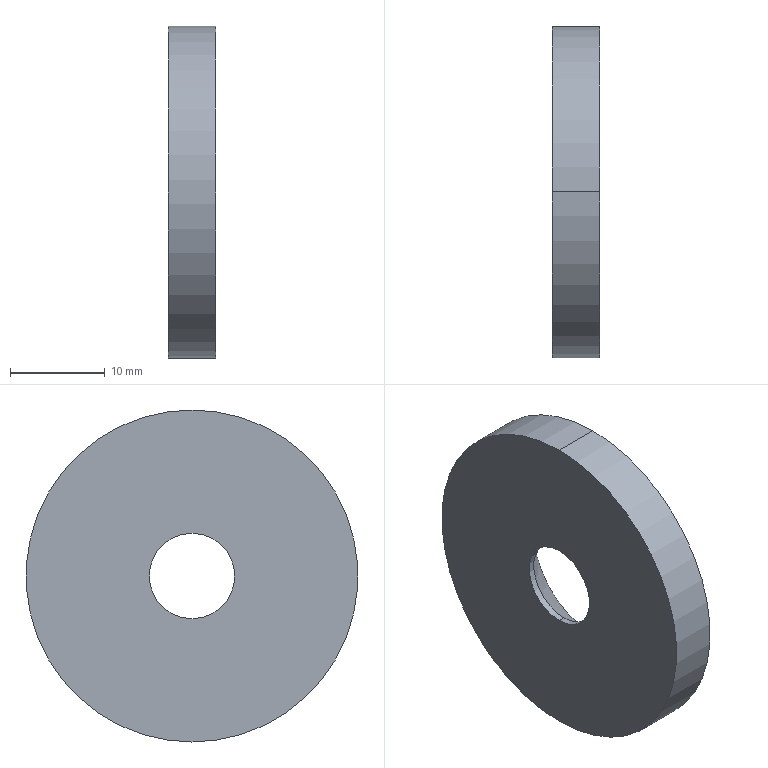Part | SolidWorks | features Extrusion 1, HoleWzd 1 | 1 solid | 8 faces | box 5 x 35 x 35 mm | volume 4148 mm3 | cylinder 4 | cone 2 | plane 2 | commonest cylinder face diameters 9 x2 35 x2
STEP:
#1=CARTESIAN_POINT('',(0.7,0.,4.5));
#2=VERTEX_POINT('',#1);
#3=CARTESIAN_POINT('',(0.7,0.,-4.5));
#4=VERTEX_POINT('',#3);
#5=CARTESIAN_POINT('',(0.7,0.,0.));
#6=DIRECTION('',(1.,0.,0.));
#7=DIRECTION('',(0.,0.,-1.));
#8=AXIS2_PLACEMENT_3D('',#5,#6,#7);
#9=CIRCLE('',#8,4.5);
#10=EDGE_CURVE('',#2,#4,#9,.T.);
#11=ORIENTED_EDGE('',*,*,#10,.F.);
#12=CARTESIAN_POINT('',(5.,0.,8.8));
#13=VERTEX_POINT('',#12);
#14=CARTESIAN_POINT('',(5.,0.,8.8));
#15=DIRECTION('',(0.7071,0.,0.7071));
#16=VECTOR('',#15,1000.);
#17=LINE('',#14,#16);
#18=EDGE_CURVE('',#2,#13,#17,.T.);
#19=ORIENTED_EDGE('',*,*,#18,.T.);
#20=CARTESIAN_POINT('',(5.,0.,-8.8));
#21=VERTEX_POINT('',#20);
#22=CARTESIAN_POINT('',(5.,0.,0.));
#23=DIRECTION('',(1.,0.,0.));
#24=DIRECTION('',(0.,0.,-1.));
#25=AXIS2_PLACEMENT_3D('',#22,#23,#24);
#26=CIRCLE('',#25,8.8);
#27=EDGE_CURVE('',#13,#21,#26,.T.);
#28=ORIENTED_EDGE('',*,*,#27,.T.);
#29=CARTESIAN_POINT('',(5.,0.,-8.8));
#30=DIRECTION('',(0.7071,0.,-0.7071));
#31=VECTOR('',#30,1000.);
#32=LINE('',#29,#31);
#33=EDGE_CURVE('',#4,#21,#32,.T.);
#34=ORIENTED_EDGE('',*,*,#33,.F.);
#35=EDGE_LOOP('',(#11,#19,#28,#34));
#36=FACE_OUTER_BOUND('',#35,.T.);
#37=CARTESIAN_POINT('',(5.,0.,0.));
#38=DIRECTION('',(1.,0.,0.));
#39=DIRECTION('',(0.,0.,-1.));
#40=AXIS2_PLACEMENT_3D('',#37,#38,#39);
#41=CONICAL_SURFACE('',#40,8.8,0.7854);
#42=ADVANCED_FACE('',(#36),#41,.F.);
#43=CARTESIAN_POINT('',(0.,0.,4.5));
#44=VERTEX_POINT('',#43);
#45=CARTESIAN_POINT('',(0.,0.,-4.5));
#46=VERTEX_POINT('',#45);
#47=CARTESIAN_POINT('',(0.,0.,0.));
#48=DIRECTION('',(1.,0.,0.));
#49=DIRECTION('',(0.,0.,-1.));
#50=AXIS2_PLACEMENT_3D('',#47,#48,#49);
#51=CIRCLE('',#50,4.5);
#52=EDGE_CURVE('',#44,#46,#51,.T.);
#53=ORIENTED_EDGE('',*,*,#52,.F.);
#54=CARTESIAN_POINT('',(5.,0.,4.5));
#55=DIRECTION('',(1.,0.,0.));
#56=VECTOR('',#55,1000.);
#57=LINE('',#54,#56);
#58=EDGE_CURVE('',#44,#2,#57,.T.);
#59=ORIENTED_EDGE('',*,*,#58,.T.);
#60=ORIENTED_EDGE('',*,*,#10,.T.);
#61=CARTESIAN_POINT('',(5.,0.,-4.5));
#62=DIRECTION('',(1.,0.,0.));
#63=VECTOR('',#62,1000.);
#64=LINE('',#61,#63);
#65=EDGE_CURVE('',#46,#4,#64,.T.);
#66=ORIENTED_EDGE('',*,*,#65,.F.);
#67=EDGE_LOOP('',(#53,#59,#60,#66));
#68=FACE_OUTER_BOUND('',#67,.T.);
#69=CARTESIAN_POINT('',(5.,0.,0.));
#70=DIRECTION('',(1.,0.,0.));
#71=DIRECTION('',(0.,0.,-1.));
#72=AXIS2_PLACEMENT_3D('',#69,#70,#71);
#73=CYLINDRICAL_SURFACE('',#72,4.5);
#74=ADVANCED_FACE('',(#68),#73,.F.);
#75=CARTESIAN_POINT('',(5.,0.,-17.5));
#76=VERTEX_POINT('',#75);
#77=CARTESIAN_POINT('',(5.,0.,17.5));
#78=VERTEX_POINT('',#77);
#79=CARTESIAN_POINT('',(5.,0.,0.));
#80=DIRECTION('',(1.,0.,0.));
#81=DIRECTION('',(0.,0.,-1.));
#82=AXIS2_PLACEMENT_3D('',#79,#80,#81);
#83=CIRCLE('',#82,17.5);
#84=EDGE_CURVE('',#76,#78,#83,.T.);
#85=ORIENTED_EDGE('',*,*,#84,.F.);
#86=CARTESIAN_POINT('',(0.,0.,-17.5));
#87=VERTEX_POINT('',#86);
#88=CARTESIAN_POINT('',(5.,0.,-17.5));
#89=DIRECTION('',(-1.,0.,0.));
#90=VECTOR('',#89,1000.);
#91=LINE('',#88,#90);
#92=EDGE_CURVE('',#76,#87,#91,.T.);
#93=ORIENTED_EDGE('',*,*,#92,.T.);
#94=CARTESIAN_POINT('',(0.,0.,17.5));
#95=VERTEX_POINT('',#94);
#96=CARTESIAN_POINT('',(0.,0.,0.));
#97=DIRECTION('',(1.,0.,0.));
#98=DIRECTION('',(0.,0.,-1.));
#99=AXIS2_PLACEMENT_3D('',#96,#97,#98);
#100=CIRCLE('',#99,17.5);
#101=EDGE_CURVE('',#87,#95,#100,.T.);
#102=ORIENTED_EDGE('',*,*,#101,.T.);
#103=CARTESIAN_POINT('',(5.,0.,17.5));
#104=DIRECTION('',(-1.,0.,0.));
#105=VECTOR('',#104,1000.);
#106=LINE('',#103,#105);
#107=EDGE_CURVE('',#78,#95,#106,.T.);
#108=ORIENTED_EDGE('',*,*,#107,.F.);
#109=EDGE_LOOP('',(#85,#93,#102,#108));
#110=FACE_OUTER_BOUND('',#109,.T.);
#111=CARTESIAN_POINT('',(5.,0.,0.));
#112=DIRECTION('',(-1.,0.,0.));
#113=DIRECTION('',(0.,0.,1.));
#114=AXIS2_PLACEMENT_3D('',#111,#112,#113);
#115=CYLINDRICAL_SURFACE('',#114,17.5);
#116=ADVANCED_FACE('',(#110),#115,.T.);
#117=ORIENTED_EDGE('',*,*,#92,.F.);
#118=CARTESIAN_POINT('',(5.,0.,0.));
#119=DIRECTION('',(1.,0.,0.));
#120=DIRECTION('',(0.,0.,-1.));
#121=AXIS2_PLACEMENT_3D('',#118,#119,#120);
#122=CIRCLE('',#121,17.5);
#123=EDGE_CURVE('',#78,#76,#122,.T.);
#124=ORIENTED_EDGE('',*,*,#123,.F.);
#125=ORIENTED_EDGE('',*,*,#107,.T.);
#126=CARTESIAN_POINT('',(0.,0.,0.));
#127=DIRECTION('',(1.,0.,0.));
#128=DIRECTION('',(0.,0.,-1.));
#129=AXIS2_PLACEMENT_3D('',#126,#127,#128);
#130=CIRCLE('',#129,17.5);
#131=EDGE_CURVE('',#95,#87,#130,.T.);
#132=ORIENTED_EDGE('',*,*,#131,.T.);
#133=EDGE_LOOP('',(#117,#124,#125,#132));
#134=FACE_OUTER_BOUND('',#133,.T.);
#135=CARTESIAN_POINT('',(5.,0.,0.));
#136=DIRECTION('',(-1.,0.,0.));
#137=DIRECTION('',(0.,0.,1.));
#138=AXIS2_PLACEMENT_3D('',#135,#136,#137);
#139=CYLINDRICAL_SURFACE('',#138,17.5);
#140=ADVANCED_FACE('',(#134),#139,.T.);
#141=CARTESIAN_POINT('',(5.,0.,0.));
#142=DIRECTION('',(1.,0.,0.));
#143=DIRECTION('',(0.,0.,-1.));
#144=AXIS2_PLACEMENT_3D('',#141,#142,#143);
#145=CIRCLE('',#144,8.8);
#146=EDGE_CURVE('',#21,#13,#145,.T.);
#147=ORIENTED_EDGE('',*,*,#146,.F.);
#148=ORIENTED_EDGE('',*,*,#27,.F.);
#149=EDGE_LOOP('',(#147,#148));
#150=FACE_BOUND('',#149,.T.);
#151=ORIENTED_EDGE('',*,*,#123,.T.);
#152=ORIENTED_EDGE('',*,*,#84,.T.);
#153=EDGE_LOOP('',(#151,#152));
#154=FACE_OUTER_BOUND('',#153,.T.);
#155=CARTESIAN_POINT('',(5.,0.,0.));
#156=DIRECTION('',(1.,0.,0.));
#157=DIRECTION('',(0.,0.,-1.));
#158=AXIS2_PLACEMENT_3D('',#155,#156,#157);
#159=PLANE('',#158);
#160=ADVANCED_FACE('',(#150,#154),#159,.T.);
#161=CARTESIAN_POINT('',(0.,0.,0.));
#162=DIRECTION('',(1.,0.,0.));
#163=DIRECTION('',(0.,0.,-1.));
#164=AXIS2_PLACEMENT_3D('',#161,#162,#163);
#165=CIRCLE('',#164,4.5);
#166=EDGE_CURVE('',#46,#44,#165,.T.);
#167=ORIENTED_EDGE('',*,*,#166,.T.);
#168=ORIENTED_EDGE('',*,*,#52,.T.);
#169=EDGE_LOOP('',(#167,#168));
#170=FACE_BOUND('',#169,.T.);
#171=ORIENTED_EDGE('',*,*,#131,.F.);
#172=ORIENTED_EDGE('',*,*,#101,.F.);
#173=EDGE_LOOP('',(#171,#172));
#174=FACE_OUTER_BOUND('',#173,.T.);
#175=CARTESIAN_POINT('',(0.,0.,0.));
#176=DIRECTION('',(1.,0.,0.));
#177=DIRECTION('',(0.,0.,-1.));
#178=AXIS2_PLACEMENT_3D('',#175,#176,#177);
#179=PLANE('',#178);
#180=ADVANCED_FACE('',(#170,#174),#179,.F.);
#181=ORIENTED_EDGE('',*,*,#58,.F.);
#182=ORIENTED_EDGE('',*,*,#166,.F.);
#183=ORIENTED_EDGE('',*,*,#65,.T.);
#184=CARTESIAN_POINT('',(0.7,0.,0.));
#185=DIRECTION('',(1.,0.,0.));
#186=DIRECTION('',(0.,0.,-1.));
#187=AXIS2_PLACEMENT_3D('',#184,#185,#186);
#188=CIRCLE('',#187,4.5);
#189=EDGE_CURVE('',#4,#2,#188,.T.);
#190=ORIENTED_EDGE('',*,*,#189,.T.);
#191=EDGE_LOOP('',(#181,#182,#183,#190));
#192=FACE_OUTER_BOUND('',#191,.T.);
#193=CARTESIAN_POINT('',(5.,0.,0.));
#194=DIRECTION('',(1.,0.,0.));
#195=DIRECTION('',(0.,0.,-1.));
#196=AXIS2_PLACEMENT_3D('',#193,#194,#195);
#197=CYLINDRICAL_SURFACE('',#196,4.5);
#198=ADVANCED_FACE('',(#192),#197,.F.);
#199=ORIENTED_EDGE('',*,*,#18,.F.);
#200=ORIENTED_EDGE('',*,*,#189,.F.);
#201=ORIENTED_EDGE('',*,*,#33,.T.);
#202=ORIENTED_EDGE('',*,*,#146,.T.);
#203=EDGE_LOOP('',(#199,#200,#201,#202));
#204=FACE_OUTER_BOUND('',#203,.T.);
#205=CARTESIAN_POINT('',(5.,0.,0.));
#206=DIRECTION('',(1.,0.,0.));
#207=DIRECTION('',(0.,0.,-1.));
#208=AXIS2_PLACEMENT_3D('',#205,#206,#207);
#209=CONICAL_SURFACE('',#208,8.8,0.7854);
#210=ADVANCED_FACE('',(#204),#209,.F.);
#211=CLOSED_SHELL('',(#42,#74,#116,#140,#160,#180,#198,#210));
#212=MANIFOLD_SOLID_BREP('',#211);
#213=CARTESIAN_POINT('',(0.,0.,0.));
#214=DIRECTION('',(0.,0.,1.));
#215=DIRECTION('',(1.,0.,0.));
#216=AXIS2_PLACEMENT_3D('',#213,#214,#215);
#217=(LENGTH_UNIT()NAMED_UNIT(*)SI_UNIT(.MILLI.,.METRE.));
#218=UNCERTAINTY_MEASURE_WITH_UNIT(LENGTH_MEASURE(0.00001),#217,'','');
#219=(NAMED_UNIT(*)PLANE_ANGLE_UNIT()SI_UNIT($,.RADIAN.));
#220=(NAMED_UNIT(*)SI_UNIT($,.STERADIAN.)SOLID_ANGLE_UNIT());
#221=(GEOMETRIC_REPRESENTATION_CONTEXT(3)GLOBAL_UNCERTAINTY_ASSIGNED_CONTEXT((#218))GLOBAL_UNIT_ASSIGNED_CONTEXT((#217,#219,#220))REPRESENTATION_CONTEXT('',''));
#222=ADVANCED_BREP_SHAPE_REPRESENTATION('',(#212,#216),#221);